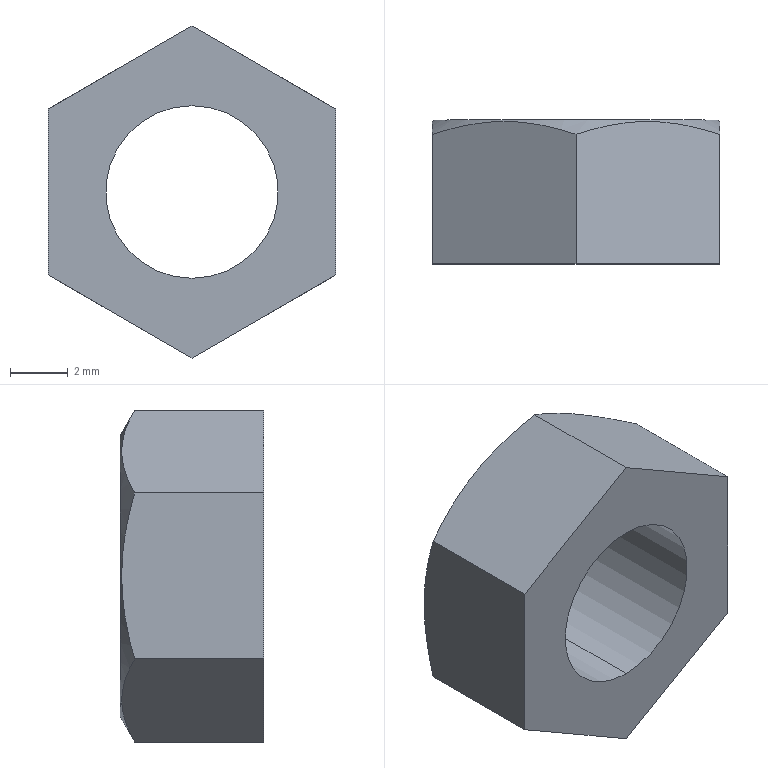Part | STEP file | NN42-M6 | 1 solid | 12 faces | box 10 x 5 x 11.547 mm | volume 289.993 mm3 | plane 8 | cylinder 2 | cone 2 | commonest cylinder face diameters 6 x2
STEP:
#1=CARTESIAN_POINT('',(0.,0.,0.));
#2=DIRECTION('',(0.,0.,1.));
#3=DIRECTION('',(1.,0.,0.));
#4=AXIS2_PLACEMENT_3D('',#1,#2,#3);
#5=CARTESIAN_POINT('',(0.,5.,-3.));
#6=VERTEX_POINT('',#5);
#7=CARTESIAN_POINT('',(0.,0.,-3.));
#8=VERTEX_POINT('',#7);
#9=CARTESIAN_POINT('',(0.,5.,-3.));
#10=DIRECTION('',(0.,-1.,0.));
#11=VECTOR('',#10,1.);
#12=LINE('',#9,#11);
#13=CARTESIAN_POINT('',(0.,5.,0.));
#14=DIRECTION('',(0.,-1.,0.));
#15=DIRECTION('',(0.,0.,-1.));
#16=AXIS2_PLACEMENT_3D('',#13,#14,#15);
#17=CYLINDRICAL_SURFACE('',#16,3.);
#18=CARTESIAN_POINT('',(6.283,0.));
#19=DIRECTION('',(0.,1.));
#20=VECTOR('',#19,1.);
#21=LINE('',#18,#20);
#22=(GEOMETRIC_REPRESENTATION_CONTEXT(2)PARAMETRIC_REPRESENTATION_CONTEXT()REPRESENTATION_CONTEXT('',''));
#23=DEFINITIONAL_REPRESENTATION('',(#21),#22);
#24=PCURVE('',#17,#23);
#25=CARTESIAN_POINT('',(0.,5.,0.));
#26=DIRECTION('',(0.,-1.,0.));
#27=DIRECTION('',(0.,0.,-1.));
#28=AXIS2_PLACEMENT_3D('',#25,#26,#27);
#29=CYLINDRICAL_SURFACE('',#28,3.);
#30=CARTESIAN_POINT('',(0.,0.));
#31=DIRECTION('',(0.,1.));
#32=VECTOR('',#31,1.);
#33=LINE('',#30,#32);
#34=(GEOMETRIC_REPRESENTATION_CONTEXT(2)PARAMETRIC_REPRESENTATION_CONTEXT()REPRESENTATION_CONTEXT('',''));
#35=DEFINITIONAL_REPRESENTATION('',(#33),#34);
#36=PCURVE('',#29,#35);
#37=SURFACE_CURVE('',#12,(#24,#36),.PCURVE_S1.);
#38=EDGE_CURVE('',#6,#8,#37,.T.);
#39=ORIENTED_EDGE('',*,*,#38,.T.);
#40=CARTESIAN_POINT('',(0.,0.,3.));
#41=VERTEX_POINT('',#40);
#42=CARTESIAN_POINT('',(0.,0.,0.));
#43=DIRECTION('',(0.,1.,0.));
#44=DIRECTION('',(0.,0.,1.));
#45=AXIS2_PLACEMENT_3D('',#42,#43,#44);
#46=CIRCLE('',#45,3.);
#47=CARTESIAN_POINT('',(9.425,5.));
#48=DIRECTION('',(-1.,0.));
#49=VECTOR('',#48,1.);
#50=LINE('',#47,#49);
#51=(GEOMETRIC_REPRESENTATION_CONTEXT(2)PARAMETRIC_REPRESENTATION_CONTEXT()REPRESENTATION_CONTEXT('',''));
#52=DEFINITIONAL_REPRESENTATION('',(#50),#51);
#53=PCURVE('',#17,#52);
#54=CARTESIAN_POINT('',(0.,0.,0.));
#55=DIRECTION('',(0.,-1.,0.));
#56=DIRECTION('',(0.,0.,1.));
#57=AXIS2_PLACEMENT_3D('',#54,#55,#56);
#58=PLANE('',#57);
#59=CARTESIAN_POINT('',(3.,0.));
#60=CARTESIAN_POINT('',(3.,-5.196));
#61=CARTESIAN_POINT('',(-1.5,-2.598));
#62=CARTESIAN_POINT('',(-6.,0.));
#63=CARTESIAN_POINT('',(-1.5,2.598));
#64=CARTESIAN_POINT('',(3.,5.196));
#65=CARTESIAN_POINT('',(3.,0.));
#66=(BOUNDED_CURVE()B_SPLINE_CURVE(2,(#59,#60,#61,#62,#63,#64,#65),.UNSPECIFIED.,.T.,.F.)B_SPLINE_CURVE_WITH_KNOTS((1,2,2,2,2,1),(-2.094,0.,2.094,4.189,6.283,8.378),.UNSPECIFIED.)CURVE()GEOMETRIC_REPRESENTATION_ITEM()RATIONAL_B_SPLINE_CURVE((1.,0.5,1.,0.5,1.,0.5,1.))REPRESENTATION_ITEM(''));
#67=(GEOMETRIC_REPRESENTATION_CONTEXT(2)PARAMETRIC_REPRESENTATION_CONTEXT()REPRESENTATION_CONTEXT('',''));
#68=DEFINITIONAL_REPRESENTATION('',(#66),#67);
#69=PCURVE('',#58,#68);
#70=SURFACE_CURVE('',#46,(#53,#69),.PCURVE_S1.);
#71=EDGE_CURVE('',#8,#41,#70,.T.);
#72=ORIENTED_EDGE('',*,*,#71,.T.);
#73=CARTESIAN_POINT('',(0.,5.,3.));
#74=VERTEX_POINT('',#73);
#75=CARTESIAN_POINT('',(0.,5.,3.));
#76=DIRECTION('',(0.,-1.,0.));
#77=VECTOR('',#76,1.);
#78=LINE('',#75,#77);
#79=CARTESIAN_POINT('',(3.142,0.));
#80=DIRECTION('',(0.,1.));
#81=VECTOR('',#80,1.);
#82=LINE('',#79,#81);
#83=(GEOMETRIC_REPRESENTATION_CONTEXT(2)PARAMETRIC_REPRESENTATION_CONTEXT()REPRESENTATION_CONTEXT('',''));
#84=DEFINITIONAL_REPRESENTATION('',(#82),#83);
#85=PCURVE('',#17,#84);
#86=CARTESIAN_POINT('',(3.142,0.));
#87=DIRECTION('',(0.,1.));
#88=VECTOR('',#87,1.);
#89=LINE('',#86,#88);
#90=(GEOMETRIC_REPRESENTATION_CONTEXT(2)PARAMETRIC_REPRESENTATION_CONTEXT()REPRESENTATION_CONTEXT('',''));
#91=DEFINITIONAL_REPRESENTATION('',(#89),#90);
#92=PCURVE('',#29,#91);
#93=SURFACE_CURVE('',#78,(#85,#92),.PCURVE_S1.);
#94=EDGE_CURVE('',#74,#41,#93,.T.);
#95=ORIENTED_EDGE('',*,*,#94,.F.);
#96=CARTESIAN_POINT('',(0.,5.,0.));
#97=DIRECTION('',(0.,-1.,0.));
#98=DIRECTION('',(0.,0.,-1.));
#99=AXIS2_PLACEMENT_3D('',#96,#97,#98);
#100=CIRCLE('',#99,3.);
#101=CARTESIAN_POINT('',(0.,0.));
#102=DIRECTION('',(1.,0.));
#103=VECTOR('',#102,1.);
#104=LINE('',#101,#103);
#105=(GEOMETRIC_REPRESENTATION_CONTEXT(2)PARAMETRIC_REPRESENTATION_CONTEXT()REPRESENTATION_CONTEXT('',''));
#106=DEFINITIONAL_REPRESENTATION('',(#104),#105);
#107=PCURVE('',#17,#106);
#108=CARTESIAN_POINT('',(0.,5.,0.));
#109=DIRECTION('',(0.,1.,0.));
#110=DIRECTION('',(-1.,0.,0.));
#111=AXIS2_PLACEMENT_3D('',#108,#109,#110);
#112=PLANE('',#111);
#113=CARTESIAN_POINT('',(0.,-3.));
#114=CARTESIAN_POINT('',(-5.196,-3.));
#115=CARTESIAN_POINT('',(-2.598,1.5));
#116=CARTESIAN_POINT('',(0.,6.));
#117=CARTESIAN_POINT('',(2.598,1.5));
#118=CARTESIAN_POINT('',(5.196,-3.));
#119=CARTESIAN_POINT('',(0.,-3.));
#120=(BOUNDED_CURVE()B_SPLINE_CURVE(2,(#113,#114,#115,#116,#117,#118,#119),.UNSPECIFIED.,.T.,.F.)B_SPLINE_CURVE_WITH_KNOTS((1,2,2,2,2,1),(-2.094,0.,2.094,4.189,6.283,8.378),.UNSPECIFIED.)CURVE()GEOMETRIC_REPRESENTATION_ITEM()RATIONAL_B_SPLINE_CURVE((1.,0.5,1.,0.5,1.,0.5,1.))REPRESENTATION_ITEM(''));
#121=(GEOMETRIC_REPRESENTATION_CONTEXT(2)PARAMETRIC_REPRESENTATION_CONTEXT()REPRESENTATION_CONTEXT('',''));
#122=DEFINITIONAL_REPRESENTATION('',(#120),#121);
#123=PCURVE('',#112,#122);
#124=SURFACE_CURVE('',#100,(#107,#123),.PCURVE_S1.);
#125=EDGE_CURVE('',#74,#6,#124,.T.);
#126=ORIENTED_EDGE('',*,*,#125,.T.);
#127=EDGE_LOOP('',(#39,#72,#95,#126));
#128=FACE_BOUND('',#127,.F.);
#129=ADVANCED_FACE('',(#128),#17,.F.);
#130=CARTESIAN_POINT('',(4.9,5.,0.));
#131=VERTEX_POINT('',#130);
#132=CARTESIAN_POINT('',(-4.9,5.,0.));
#133=VERTEX_POINT('',#132);
#134=CARTESIAN_POINT('',(0.,5.,0.));
#135=DIRECTION('',(0.,-1.,0.));
#136=DIRECTION('',(1.,0.,0.));
#137=AXIS2_PLACEMENT_3D('',#134,#135,#136);
#138=CIRCLE('',#137,4.9);
#139=CARTESIAN_POINT('',(0.,5.,0.));
#140=DIRECTION('',(0.,-1.,0.));
#141=DIRECTION('',(1.,0.,0.));
#142=AXIS2_PLACEMENT_3D('',#139,#140,#141);
#143=CONICAL_SURFACE('',#142,4.9,1.047);
#144=CARTESIAN_POINT('',(0.,0.));
#145=DIRECTION('',(1.,0.));
#146=VECTOR('',#145,1.);
#147=LINE('',#144,#146);
#148=(GEOMETRIC_REPRESENTATION_CONTEXT(2)PARAMETRIC_REPRESENTATION_CONTEXT()REPRESENTATION_CONTEXT('',''));
#149=DEFINITIONAL_REPRESENTATION('',(#147),#148);
#150=PCURVE('',#143,#149);
#151=CARTESIAN_POINT('',(-4.9,0.));
#152=CARTESIAN_POINT('',(-4.9,8.487));
#153=CARTESIAN_POINT('',(2.45,4.244));
#154=CARTESIAN_POINT('',(9.8,0.));
#155=CARTESIAN_POINT('',(2.45,-4.244));
#156=CARTESIAN_POINT('',(-4.9,-8.487));
#157=CARTESIAN_POINT('',(-4.9,0.));
#158=(BOUNDED_CURVE()B_SPLINE_CURVE(2,(#151,#152,#153,#154,#155,#156,#157),.UNSPECIFIED.,.T.,.F.)B_SPLINE_CURVE_WITH_KNOTS((1,2,2,2,2,1),(-2.094,0.,2.094,4.189,6.283,8.378),.UNSPECIFIED.)CURVE()GEOMETRIC_REPRESENTATION_ITEM()RATIONAL_B_SPLINE_CURVE((1.,0.5,1.,0.5,1.,0.5,1.))REPRESENTATION_ITEM(''));
#159=(GEOMETRIC_REPRESENTATION_CONTEXT(2)PARAMETRIC_REPRESENTATION_CONTEXT()REPRESENTATION_CONTEXT('',''));
#160=DEFINITIONAL_REPRESENTATION('',(#158),#159);
#161=PCURVE('',#112,#160);
#162=SURFACE_CURVE('',#138,(#150,#161),.PCURVE_S1.);
#163=EDGE_CURVE('',#131,#133,#162,.T.);
#164=ORIENTED_EDGE('',*,*,#163,.T.);
#165=CARTESIAN_POINT('',(-5.,4.942,0.));
#166=VERTEX_POINT('',#165);
#167=CARTESIAN_POINT('',(-4.9,5.,0.));
#168=DIRECTION('',(-0.866,-0.5,0.));
#169=VECTOR('',#168,1.);
#170=LINE('',#167,#169);
#171=CARTESIAN_POINT('',(3.142,0.));
#172=DIRECTION('',(0.,1.));
#173=VECTOR('',#172,1.);
#174=LINE('',#171,#173);
#175=(GEOMETRIC_REPRESENTATION_CONTEXT(2)PARAMETRIC_REPRESENTATION_CONTEXT()REPRESENTATION_CONTEXT('',''));
#176=DEFINITIONAL_REPRESENTATION('',(#174),#175);
#177=PCURVE('',#143,#176);
#178=CARTESIAN_POINT('',(0.,5.,0.));
#179=DIRECTION('',(0.,-1.,0.));
#180=DIRECTION('',(1.,0.,0.));
#181=AXIS2_PLACEMENT_3D('',#178,#179,#180);
#182=CONICAL_SURFACE('',#181,4.9,1.047);
#183=CARTESIAN_POINT('',(3.142,0.));
#184=DIRECTION('',(0.,1.));
#185=VECTOR('',#184,1.);
#186=LINE('',#183,#185);
#187=(GEOMETRIC_REPRESENTATION_CONTEXT(2)PARAMETRIC_REPRESENTATION_CONTEXT()REPRESENTATION_CONTEXT('',''));
#188=DEFINITIONAL_REPRESENTATION('',(#186),#187);
#189=PCURVE('',#182,#188);
#190=SURFACE_CURVE('',#170,(#177,#189),.PCURVE_S1.);
#191=EDGE_CURVE('',#133,#166,#190,.T.);
#192=ORIENTED_EDGE('',*,*,#191,.T.);
#193=CARTESIAN_POINT('',(-5.,4.496,2.887));
#194=VERTEX_POINT('',#193);
#195=CARTESIAN_POINT('',(-5.,4.496,2.887));
#196=CARTESIAN_POINT('',(-5.,4.767,1.946));
#197=CARTESIAN_POINT('',(-5.,4.942,0.9887));
#198=CARTESIAN_POINT('',(-5.,4.942,0.));
#199=B_SPLINE_CURVE_WITH_KNOTS('',3,(#195,#196,#197,#198),.UNSPECIFIED.,.F.,.F.,(4,4),(0.006295,0.009232),.PIECEWISE_BEZIER_KNOTS.);
#200=CARTESIAN_POINT('',(2.618,0.5043));
#201=CARTESIAN_POINT('',(2.624,0.492));
#202=CARTESIAN_POINT('',(2.637,0.4677));
#203=CARTESIAN_POINT('',(2.657,0.4325));
#204=CARTESIAN_POINT('',(2.678,0.3985));
#205=CARTESIAN_POINT('',(2.699,0.3659));
#206=CARTESIAN_POINT('',(2.72,0.3347));
#207=CARTESIAN_POINT('',(2.742,0.3048));
#208=CARTESIAN_POINT('',(2.764,0.2764));
#209=CARTESIAN_POINT('',(2.787,0.2495));
#210=CARTESIAN_POINT('',(2.81,0.2242));
#211=CARTESIAN_POINT('',(2.833,0.2005));
#212=CARTESIAN_POINT('',(2.857,0.1784));
#213=CARTESIAN_POINT('',(2.882,0.158));
#214=CARTESIAN_POINT('',(2.906,0.1394));
#215=CARTESIAN_POINT('',(2.931,0.1226));
#216=CARTESIAN_POINT('',(2.957,0.1076));
#217=CARTESIAN_POINT('',(2.982,0.09448));
#218=CARTESIAN_POINT('',(3.008,0.08328));
#219=CARTESIAN_POINT('',(3.035,0.07404));
#220=CARTESIAN_POINT('',(3.061,0.0668));
#221=CARTESIAN_POINT('',(3.088,0.06159));
#222=CARTESIAN_POINT('',(3.115,0.05844));
#223=CARTESIAN_POINT('',(3.133,0.05773));
#224=CARTESIAN_POINT('',(3.142,0.05774));
#225=B_SPLINE_CURVE_WITH_KNOTS('',3,(#200,#201,#202,#203,#204,#205,#206,#207,#208,#209,#210,#211,#212,#213,#214,#215,#216,#217,#218,#219,#220,#221,#222,#223,#224),.UNSPECIFIED.,.F.,.F.,(4,1,1,1,1,1,1,1,1,1,1,1,1,1,1,1,1,1,1,1,1,1,4),(0.006295,0.006428,0.006562,0.006695,0.006829,0.006962,0.007096,0.007229,0.007363,0.007496,0.00763,0.007763,0.007897,0.00803,0.008164,0.008297,0.008431,0.008564,0.008698,0.008831,0.008965,0.009098,0.009232),.QUASI_UNIFORM_KNOTS.);
#226=(GEOMETRIC_REPRESENTATION_CONTEXT(2)PARAMETRIC_REPRESENTATION_CONTEXT()REPRESENTATION_CONTEXT('',''));
#227=DEFINITIONAL_REPRESENTATION('',(#225),#226);
#228=PCURVE('',#143,#227);
#229=CARTESIAN_POINT('',(-5.,4.496,2.887));
#230=DIRECTION('',(1.,0.,0.));
#231=DIRECTION('',(0.,0.,1.));
#232=AXIS2_PLACEMENT_3D('',#229,#230,#231);
#233=PLANE('',#232);
#234=CARTESIAN_POINT('',(0.,0.));
#235=CARTESIAN_POINT('',(-0.9405,-0.2715));
#236=CARTESIAN_POINT('',(-1.898,-0.4466));
#237=CARTESIAN_POINT('',(-2.887,-0.4466));
#238=B_SPLINE_CURVE_WITH_KNOTS('',3,(#234,#235,#236,#237),.UNSPECIFIED.,.F.,.F.,(4,4),(0.006295,0.009232),.PIECEWISE_BEZIER_KNOTS.);
#239=(GEOMETRIC_REPRESENTATION_CONTEXT(2)PARAMETRIC_REPRESENTATION_CONTEXT()REPRESENTATION_CONTEXT('',''));
#240=DEFINITIONAL_REPRESENTATION('',(#238),#239);
#241=PCURVE('',#233,#240);
#242=SURFACE_CURVE('',#199,(#228,#241),.PCURVE_S1.);
#243=EDGE_CURVE('',#194,#166,#242,.T.);
#244=ORIENTED_EDGE('',*,*,#243,.F.);
#245=CARTESIAN_POINT('',(0.,4.496,5.774));
#246=VERTEX_POINT('',#245);
#247=CARTESIAN_POINT('',(0.,4.496,5.774));
#248=CARTESIAN_POINT('',(-0.8164,4.768,5.302));
#249=CARTESIAN_POINT('',(-1.645,4.942,4.824));
#250=CARTESIAN_POINT('',(-2.708,4.942,4.21));
#251=CARTESIAN_POINT('',(-2.921,4.932,4.087));
#252=CARTESIAN_POINT('',(-3.344,4.891,3.843));
#253=CARTESIAN_POINT('',(-3.554,4.861,3.722));
#254=CARTESIAN_POINT('',(-4.179,4.744,3.361));
#255=CARTESIAN_POINT('',(-4.591,4.632,3.123));
#256=CARTESIAN_POINT('',(-5.,4.496,2.887));
#257=B_SPLINE_CURVE_WITH_KNOTS('',3,(#247,#248,#249,#250,#251,#252,#253,#254,#255,#256),.UNSPECIFIED.,.F.,.F.,(4,2,2,2,4),(0.000000238,0.002916,0.003645,0.004373,0.005831),.UNSPECIFIED.);
#258=CARTESIAN_POINT('',(1.571,0.5043));
#259=CARTESIAN_POINT('',(1.584,0.4796));
#260=CARTESIAN_POINT('',(1.61,0.4317));
#261=CARTESIAN_POINT('',(1.651,0.365));
#262=CARTESIAN_POINT('',(1.694,0.3038));
#263=CARTESIAN_POINT('',(1.739,0.2486));
#264=CARTESIAN_POINT('',(1.786,0.1995));
#265=CARTESIAN_POINT('',(1.834,0.1571));
#266=CARTESIAN_POINT('',(1.884,0.1217));
#267=CARTESIAN_POINT('',(1.935,0.09364));
#268=CARTESIAN_POINT('',(1.987,0.07321));
#269=CARTESIAN_POINT('',(2.04,0.06069));
#270=CARTESIAN_POINT('',(2.093,0.05635));
#271=CARTESIAN_POINT('',(2.147,0.06034));
#272=CARTESIAN_POINT('',(2.2,0.07259));
#273=CARTESIAN_POINT('',(2.253,0.09288));
#274=CARTESIAN_POINT('',(2.304,0.1209));
#275=CARTESIAN_POINT('',(2.354,0.1563));
#276=CARTESIAN_POINT('',(2.402,0.1988));
#277=CARTESIAN_POINT('',(2.449,0.248));
#278=CARTESIAN_POINT('',(2.494,0.3034));
#279=CARTESIAN_POINT('',(2.537,0.3648));
#280=CARTESIAN_POINT('',(2.579,0.4316));
#281=CARTESIAN_POINT('',(2.605,0.4795));
#282=CARTESIAN_POINT('',(2.618,0.5043));
#283=B_SPLINE_CURVE_WITH_KNOTS('',3,(#258,#259,#260,#261,#262,#263,#264,#265,#266,#267,#268,#269,#270,#271,#272,#273,#274,#275,#276,#277,#278,#279,#280,#281,#282),.UNSPECIFIED.,.F.,.F.,(4,1,1,1,1,1,1,1,1,1,1,1,1,1,1,1,1,1,1,1,1,1,4),(0.000000238,0.0002653,0.0005303,0.0007954,0.00106,0.001325,0.00159,0.001856,0.002121,0.002386,0.002651,0.002916,0.003181,0.003446,0.003711,0.003976,0.004241,0.004506,0.004771,0.005036,0.005301,0.005566,0.005831),.QUASI_UNIFORM_KNOTS.);
#284=(GEOMETRIC_REPRESENTATION_CONTEXT(2)PARAMETRIC_REPRESENTATION_CONTEXT()REPRESENTATION_CONTEXT('',''));
#285=DEFINITIONAL_REPRESENTATION('',(#283),#284);
#286=PCURVE('',#143,#285);
#287=CARTESIAN_POINT('',(0.,4.496,5.774));
#288=DIRECTION('',(0.5,0.,-0.866));
#289=DIRECTION('',(0.866,0.,0.5));
#290=AXIS2_PLACEMENT_3D('',#287,#288,#289);
#291=PLANE('',#290);
#292=CARTESIAN_POINT('',(0.,0.));
#293=CARTESIAN_POINT('',(-0.9427,-0.2721));
#294=CARTESIAN_POINT('',(-1.9,-0.446));
#295=CARTESIAN_POINT('',(-3.127,-0.4467));
#296=CARTESIAN_POINT('',(-3.373,-0.4363));
#297=CARTESIAN_POINT('',(-3.861,-0.3956));
#298=CARTESIAN_POINT('',(-4.103,-0.3654));
#299=CARTESIAN_POINT('',(-4.826,-0.2487));
#300=CARTESIAN_POINT('',(-5.302,-0.1362));
#301=CARTESIAN_POINT('',(-5.774,0.));
#302=B_SPLINE_CURVE_WITH_KNOTS('',3,(#292,#293,#294,#295,#296,#297,#298,#299,#300,#301),.UNSPECIFIED.,.F.,.F.,(4,2,2,2,4),(0.000000238,0.002916,0.003645,0.004373,0.005831),.UNSPECIFIED.);
#303=(GEOMETRIC_REPRESENTATION_CONTEXT(2)PARAMETRIC_REPRESENTATION_CONTEXT()REPRESENTATION_CONTEXT('',''));
#304=DEFINITIONAL_REPRESENTATION('',(#302),#303);
#305=PCURVE('',#291,#304);
#306=SURFACE_CURVE('',#257,(#286,#305),.PCURVE_S1.);
#307=EDGE_CURVE('',#246,#194,#306,.T.);
#308=ORIENTED_EDGE('',*,*,#307,.F.);
#309=CARTESIAN_POINT('',(5.,4.496,2.887));
#310=VERTEX_POINT('',#309);
#311=CARTESIAN_POINT('',(5.,4.496,2.887));
#312=CARTESIAN_POINT('',(4.184,4.768,3.358));
#313=CARTESIAN_POINT('',(3.355,4.942,3.837));
#314=CARTESIAN_POINT('',(2.292,4.942,4.45));
#315=CARTESIAN_POINT('',(2.079,4.932,4.573));
#316=CARTESIAN_POINT('',(1.656,4.891,4.817));
#317=CARTESIAN_POINT('',(1.446,4.861,4.938));
#318=CARTESIAN_POINT('',(0.8208,4.744,5.3));
#319=CARTESIAN_POINT('',(0.4087,4.632,5.538));
#320=CARTESIAN_POINT('',(0.,4.496,5.774));
#321=B_SPLINE_CURVE_WITH_KNOTS('',3,(#311,#312,#313,#314,#315,#316,#317,#318,#319,#320),.UNSPECIFIED.,.F.,.F.,(4,2,2,2,4),(0.000000238,0.002916,0.003645,0.004373,0.005831),.UNSPECIFIED.);
#322=CARTESIAN_POINT('',(0.5236,0.5043));
#323=CARTESIAN_POINT('',(0.5365,0.4796));
#324=CARTESIAN_POINT('',(0.5628,0.4317));
#325=CARTESIAN_POINT('',(0.6041,0.365));
#326=CARTESIAN_POINT('',(0.6472,0.3038));
#327=CARTESIAN_POINT('',(0.6921,0.2486));
#328=CARTESIAN_POINT('',(0.7388,0.1995));
#329=CARTESIAN_POINT('',(0.787,0.1571));
#330=CARTESIAN_POINT('',(0.8367,0.1217));
#331=CARTESIAN_POINT('',(0.8877,0.09364));
#332=CARTESIAN_POINT('',(0.9398,0.07321));
#333=CARTESIAN_POINT('',(0.9926,0.06069));
#334=CARTESIAN_POINT('',(1.046,0.05635));
#335=CARTESIAN_POINT('',(1.1,0.06034));
#336=CARTESIAN_POINT('',(1.153,0.07259));
#337=CARTESIAN_POINT('',(1.205,0.09288));
#338=CARTESIAN_POINT('',(1.257,0.1209));
#339=CARTESIAN_POINT('',(1.307,0.1563));
#340=CARTESIAN_POINT('',(1.355,0.1988));
#341=CARTESIAN_POINT('',(1.402,0.248));
#342=CARTESIAN_POINT('',(1.447,0.3034));
#343=CARTESIAN_POINT('',(1.49,0.3648));
#344=CARTESIAN_POINT('',(1.532,0.4316));
#345=CARTESIAN_POINT('',(1.558,0.4795));
#346=CARTESIAN_POINT('',(1.571,0.5043));
#347=B_SPLINE_CURVE_WITH_KNOTS('',3,(#322,#323,#324,#325,#326,#327,#328,#329,#330,#331,#332,#333,#334,#335,#336,#337,#338,#339,#340,#341,#342,#343,#344,#345,#346),.UNSPECIFIED.,.F.,.F.,(4,1,1,1,1,1,1,1,1,1,1,1,1,1,1,1,1,1,1,1,1,1,4),(0.000000238,0.0002653,0.0005303,0.0007954,0.00106,0.001325,0.00159,0.001856,0.002121,0.002386,0.002651,0.002916,0.003181,0.003446,0.003711,0.003976,0.004241,0.004506,0.004771,0.005036,0.005301,0.005566,0.005831),.QUASI_UNIFORM_KNOTS.);
#348=(GEOMETRIC_REPRESENTATION_CONTEXT(2)PARAMETRIC_REPRESENTATION_CONTEXT()REPRESENTATION_CONTEXT('',''));
#349=DEFINITIONAL_REPRESENTATION('',(#347),#348);
#350=PCURVE('',#143,#349);
#351=CARTESIAN_POINT('',(5.,4.496,2.887));
#352=DIRECTION('',(-0.5,0.,-0.866));
#353=DIRECTION('',(0.866,0.,-0.5));
#354=AXIS2_PLACEMENT_3D('',#351,#352,#353);
#355=PLANE('',#354);
#356=CARTESIAN_POINT('',(0.,0.));
#357=CARTESIAN_POINT('',(-0.9427,-0.2721));
#358=CARTESIAN_POINT('',(-1.9,-0.446));
#359=CARTESIAN_POINT('',(-3.127,-0.4467));
#360=CARTESIAN_POINT('',(-3.373,-0.4363));
#361=CARTESIAN_POINT('',(-3.861,-0.3956));
#362=CARTESIAN_POINT('',(-4.103,-0.3654));
#363=CARTESIAN_POINT('',(-4.826,-0.2487));
#364=CARTESIAN_POINT('',(-5.302,-0.1362));
#365=CARTESIAN_POINT('',(-5.774,0.));
#366=B_SPLINE_CURVE_WITH_KNOTS('',3,(#356,#357,#358,#359,#360,#361,#362,#363,#364,#365),.UNSPECIFIED.,.F.,.F.,(4,2,2,2,4),(0.000000238,0.002916,0.003645,0.004373,0.005831),.UNSPECIFIED.);
#367=(GEOMETRIC_REPRESENTATION_CONTEXT(2)PARAMETRIC_REPRESENTATION_CONTEXT()REPRESENTATION_CONTEXT('',''));
#368=DEFINITIONAL_REPRESENTATION('',(#366),#367);
#369=PCURVE('',#355,#368);
#370=SURFACE_CURVE('',#321,(#350,#369),.PCURVE_S1.);
#371=EDGE_CURVE('',#310,#246,#370,.T.);
#372=ORIENTED_EDGE('',*,*,#371,.F.);
#373=CARTESIAN_POINT('',(5.,4.942,0.));
#374=VERTEX_POINT('',#373);
#375=CARTESIAN_POINT('',(5.,4.942,0.));
#376=CARTESIAN_POINT('',(5.,4.942,0.4941));
#377=CARTESIAN_POINT('',(5.,4.899,0.982));
#378=CARTESIAN_POINT('',(5.,4.743,1.943));
#379=CARTESIAN_POINT('',(5.,4.631,2.417));
#380=CARTESIAN_POINT('',(5.,4.496,2.887));
#381=B_SPLINE_CURVE_WITH_KNOTS('',3,(#375,#376,#377,#378,#379,#380),.UNSPECIFIED.,.F.,.F.,(4,2,4),(0.009232,0.0107,0.01217),.UNSPECIFIED.);
#382=CARTESIAN_POINT('',(0.,0.05774));
#383=CARTESIAN_POINT('',(0.008983,0.05773));
#384=CARTESIAN_POINT('',(0.02693,0.05844));
#385=CARTESIAN_POINT('',(0.05375,0.06158));
#386=CARTESIAN_POINT('',(0.08042,0.06677));
#387=CARTESIAN_POINT('',(0.1069,0.074));
#388=CARTESIAN_POINT('',(0.1332,0.08323));
#389=CARTESIAN_POINT('',(0.1592,0.09442));
#390=CARTESIAN_POINT('',(0.185,0.1075));
#391=CARTESIAN_POINT('',(0.2104,0.1225));
#392=CARTESIAN_POINT('',(0.2355,0.1394));
#393=CARTESIAN_POINT('',(0.2603,0.158));
#394=CARTESIAN_POINT('',(0.2846,0.1784));
#395=CARTESIAN_POINT('',(0.3086,0.2005));
#396=CARTESIAN_POINT('',(0.3321,0.2242));
#397=CARTESIAN_POINT('',(0.3552,0.2496));
#398=CARTESIAN_POINT('',(0.3779,0.2765));
#399=CARTESIAN_POINT('',(0.4001,0.3049));
#400=CARTESIAN_POINT('',(0.4218,0.3347));
#401=CARTESIAN_POINT('',(0.4431,0.366));
#402=CARTESIAN_POINT('',(0.464,0.3986));
#403=CARTESIAN_POINT('',(0.4843,0.4325));
#404=CARTESIAN_POINT('',(0.5042,0.4677));
#405=CARTESIAN_POINT('',(0.5172,0.492));
#406=CARTESIAN_POINT('',(0.5236,0.5043));
#407=B_SPLINE_CURVE_WITH_KNOTS('',3,(#382,#383,#384,#385,#386,#387,#388,#389,#390,#391,#392,#393,#394,#395,#396,#397,#398,#399,#400,#401,#402,#403,#404,#405,#406),.UNSPECIFIED.,.F.,.F.,(4,1,1,1,1,1,1,1,1,1,1,1,1,1,1,1,1,1,1,1,1,1,4),(0.009232,0.009365,0.009499,0.009632,0.009765,0.009899,0.01003,0.01017,0.0103,0.01043,0.01057,0.0107,0.01083,0.01097,0.0111,0.01123,0.01137,0.0115,0.01163,0.01177,0.0119,0.01203,0.01217),.QUASI_UNIFORM_KNOTS.);
#408=(GEOMETRIC_REPRESENTATION_CONTEXT(2)PARAMETRIC_REPRESENTATION_CONTEXT()REPRESENTATION_CONTEXT('',''));
#409=DEFINITIONAL_REPRESENTATION('',(#407),#408);
#410=PCURVE('',#143,#409);
#411=CARTESIAN_POINT('',(5.,4.496,-2.887));
#412=DIRECTION('',(-1.,0.,0.));
#413=DIRECTION('',(0.,0.,-1.));
#414=AXIS2_PLACEMENT_3D('',#411,#412,#413);
#415=PLANE('',#414);
#416=CARTESIAN_POINT('',(-2.887,-0.4466));
#417=CARTESIAN_POINT('',(-3.381,-0.4466));
#418=CARTESIAN_POINT('',(-3.869,-0.4035));
#419=CARTESIAN_POINT('',(-4.83,-0.2477));
#420=CARTESIAN_POINT('',(-5.304,-0.1356));
#421=CARTESIAN_POINT('',(-5.774,0.));
#422=B_SPLINE_CURVE_WITH_KNOTS('',3,(#416,#417,#418,#419,#420,#421),.UNSPECIFIED.,.F.,.F.,(4,2,4),(0.009232,0.0107,0.01217),.UNSPECIFIED.);
#423=(GEOMETRIC_REPRESENTATION_CONTEXT(2)PARAMETRIC_REPRESENTATION_CONTEXT()REPRESENTATION_CONTEXT('',''));
#424=DEFINITIONAL_REPRESENTATION('',(#422),#423);
#425=PCURVE('',#415,#424);
#426=SURFACE_CURVE('',#381,(#410,#425),.PCURVE_S1.);
#427=EDGE_CURVE('',#374,#310,#426,.T.);
#428=ORIENTED_EDGE('',*,*,#427,.F.);
#429=CARTESIAN_POINT('',(4.9,5.,0.));
#430=DIRECTION('',(0.866,-0.5,0.));
#431=VECTOR('',#430,1.);
#432=LINE('',#429,#431);
#433=CARTESIAN_POINT('',(0.,0.));
#434=DIRECTION('',(0.,1.));
#435=VECTOR('',#434,1.);
#436=LINE('',#433,#435);
#437=(GEOMETRIC_REPRESENTATION_CONTEXT(2)PARAMETRIC_REPRESENTATION_CONTEXT()REPRESENTATION_CONTEXT('',''));
#438=DEFINITIONAL_REPRESENTATION('',(#436),#437);
#439=PCURVE('',#143,#438);
#440=CARTESIAN_POINT('',(6.283,0.));
#441=DIRECTION('',(0.,1.));
#442=VECTOR('',#441,1.);
#443=LINE('',#440,#442);
#444=(GEOMETRIC_REPRESENTATION_CONTEXT(2)PARAMETRIC_REPRESENTATION_CONTEXT()REPRESENTATION_CONTEXT('',''));
#445=DEFINITIONAL_REPRESENTATION('',(#443),#444);
#446=PCURVE('',#182,#445);
#447=SURFACE_CURVE('',#432,(#439,#446),.PCURVE_S1.);
#448=EDGE_CURVE('',#131,#374,#447,.T.);
#449=ORIENTED_EDGE('',*,*,#448,.F.);
#450=EDGE_LOOP('',(#164,#192,#244,#308,#372,#428,#449));
#451=FACE_BOUND('',#450,.T.);
#452=ADVANCED_FACE('',(#451),#143,.T.);
#453=ORIENTED_EDGE('',*,*,#191,.F.);
#454=CARTESIAN_POINT('',(0.,5.,0.));
#455=DIRECTION('',(0.,-1.,0.));
#456=DIRECTION('',(1.,0.,0.));
#457=AXIS2_PLACEMENT_3D('',#454,#455,#456);
#458=CIRCLE('',#457,4.9);
#459=CARTESIAN_POINT('',(0.,0.));
#460=DIRECTION('',(1.,0.));
#461=VECTOR('',#460,1.);
#462=LINE('',#459,#461);
#463=(GEOMETRIC_REPRESENTATION_CONTEXT(2)PARAMETRIC_REPRESENTATION_CONTEXT()REPRESENTATION_CONTEXT('',''));
#464=DEFINITIONAL_REPRESENTATION('',(#462),#463);
#465=PCURVE('',#182,#464);
#466=CARTESIAN_POINT('',(-4.9,0.));
#467=CARTESIAN_POINT('',(-4.9,8.487));
#468=CARTESIAN_POINT('',(2.45,4.244));
#469=CARTESIAN_POINT('',(9.8,0.));
#470=CARTESIAN_POINT('',(2.45,-4.244));
#471=CARTESIAN_POINT('',(-4.9,-8.487));
#472=CARTESIAN_POINT('',(-4.9,0.));
#473=(BOUNDED_CURVE()B_SPLINE_CURVE(2,(#466,#467,#468,#469,#470,#471,#472),.UNSPECIFIED.,.T.,.F.)B_SPLINE_CURVE_WITH_KNOTS((1,2,2,2,2,1),(-2.094,0.,2.094,4.189,6.283,8.378),.UNSPECIFIED.)CURVE()GEOMETRIC_REPRESENTATION_ITEM()RATIONAL_B_SPLINE_CURVE((1.,0.5,1.,0.5,1.,0.5,1.))REPRESENTATION_ITEM(''));
#474=(GEOMETRIC_REPRESENTATION_CONTEXT(2)PARAMETRIC_REPRESENTATION_CONTEXT()REPRESENTATION_CONTEXT('',''));
#475=DEFINITIONAL_REPRESENTATION('',(#473),#474);
#476=PCURVE('',#112,#475);
#477=SURFACE_CURVE('',#458,(#465,#476),.PCURVE_S1.);
#478=EDGE_CURVE('',#133,#131,#477,.T.);
#479=ORIENTED_EDGE('',*,*,#478,.T.);
#480=ORIENTED_EDGE('',*,*,#448,.T.);
#481=CARTESIAN_POINT('',(5.,4.496,-2.887));
#482=VERTEX_POINT('',#481);
#483=CARTESIAN_POINT('',(5.,4.496,-2.887));
#484=CARTESIAN_POINT('',(5.,4.767,-1.946));
#485=CARTESIAN_POINT('',(5.,4.942,-0.9887));
#486=CARTESIAN_POINT('',(5.,4.942,0.));
#487=B_SPLINE_CURVE_WITH_KNOTS('',3,(#483,#484,#485,#486),.UNSPECIFIED.,.F.,.F.,(4,4),(0.006295,0.009232),.PIECEWISE_BEZIER_KNOTS.);
#488=CARTESIAN_POINT('',(5.76,0.5043));
#489=CARTESIAN_POINT('',(5.766,0.492));
#490=CARTESIAN_POINT('',(5.779,0.4677));
#491=CARTESIAN_POINT('',(5.799,0.4325));
#492=CARTESIAN_POINT('',(5.819,0.3985));
#493=CARTESIAN_POINT('',(5.84,0.3659));
#494=CARTESIAN_POINT('',(5.861,0.3347));
#495=CARTESIAN_POINT('',(5.883,0.3048));
#496=CARTESIAN_POINT('',(5.905,0.2764));
#497=CARTESIAN_POINT('',(5.928,0.2495));
#498=CARTESIAN_POINT('',(5.951,0.2242));
#499=CARTESIAN_POINT('',(5.975,0.2005));
#500=CARTESIAN_POINT('',(5.999,0.1784));
#501=CARTESIAN_POINT('',(6.023,0.158));
#502=CARTESIAN_POINT('',(6.048,0.1394));
#503=CARTESIAN_POINT('',(6.073,0.1226));
#504=CARTESIAN_POINT('',(6.098,0.1076));
#505=CARTESIAN_POINT('',(6.124,0.09448));
#506=CARTESIAN_POINT('',(6.15,0.08328));
#507=CARTESIAN_POINT('',(6.176,0.07404));
#508=CARTESIAN_POINT('',(6.203,0.0668));
#509=CARTESIAN_POINT('',(6.229,0.06159));
#510=CARTESIAN_POINT('',(6.256,0.05844));
#511=CARTESIAN_POINT('',(6.274,0.05773));
#512=CARTESIAN_POINT('',(6.283,0.05774));
#513=B_SPLINE_CURVE_WITH_KNOTS('',3,(#488,#489,#490,#491,#492,#493,#494,#495,#496,#497,#498,#499,#500,#501,#502,#503,#504,#505,#506,#507,#508,#509,#510,#511,#512),.UNSPECIFIED.,.F.,.F.,(4,1,1,1,1,1,1,1,1,1,1,1,1,1,1,1,1,1,1,1,1,1,4),(0.006295,0.006428,0.006562,0.006695,0.006829,0.006962,0.007096,0.007229,0.007363,0.007496,0.00763,0.007763,0.007897,0.00803,0.008164,0.008297,0.008431,0.008564,0.008698,0.008831,0.008965,0.009098,0.009232),.QUASI_UNIFORM_KNOTS.);
#514=(GEOMETRIC_REPRESENTATION_CONTEXT(2)PARAMETRIC_REPRESENTATION_CONTEXT()REPRESENTATION_CONTEXT('',''));
#515=DEFINITIONAL_REPRESENTATION('',(#513),#514);
#516=PCURVE('',#182,#515);
#517=CARTESIAN_POINT('',(0.,0.));
#518=CARTESIAN_POINT('',(-0.9405,-0.2715));
#519=CARTESIAN_POINT('',(-1.898,-0.4466));
#520=CARTESIAN_POINT('',(-2.887,-0.4466));
#521=B_SPLINE_CURVE_WITH_KNOTS('',3,(#517,#518,#519,#520),.UNSPECIFIED.,.F.,.F.,(4,4),(0.006295,0.009232),.PIECEWISE_BEZIER_KNOTS.);
#522=(GEOMETRIC_REPRESENTATION_CONTEXT(2)PARAMETRIC_REPRESENTATION_CONTEXT()REPRESENTATION_CONTEXT('',''));
#523=DEFINITIONAL_REPRESENTATION('',(#521),#522);
#524=PCURVE('',#415,#523);
#525=SURFACE_CURVE('',#487,(#516,#524),.PCURVE_S1.);
#526=EDGE_CURVE('',#482,#374,#525,.T.);
#527=ORIENTED_EDGE('',*,*,#526,.F.);
#528=CARTESIAN_POINT('',(0.,4.496,-5.774));
#529=VERTEX_POINT('',#528);
#530=CARTESIAN_POINT('',(0.,4.496,-5.774));
#531=CARTESIAN_POINT('',(0.8164,4.768,-5.302));
#532=CARTESIAN_POINT('',(1.645,4.942,-4.824));
#533=CARTESIAN_POINT('',(2.708,4.942,-4.21));
#534=CARTESIAN_POINT('',(2.921,4.932,-4.087));
#535=CARTESIAN_POINT('',(3.344,4.891,-3.843));
#536=CARTESIAN_POINT('',(3.554,4.861,-3.722));
#537=CARTESIAN_POINT('',(4.179,4.744,-3.361));
#538=CARTESIAN_POINT('',(4.591,4.632,-3.123));
#539=CARTESIAN_POINT('',(5.,4.496,-2.887));
#540=B_SPLINE_CURVE_WITH_KNOTS('',3,(#530,#531,#532,#533,#534,#535,#536,#537,#538,#539),.UNSPECIFIED.,.F.,.F.,(4,2,2,2,4),(0.000000238,0.002916,0.003645,0.004373,0.005831),.UNSPECIFIED.);
#541=CARTESIAN_POINT('',(4.712,0.5043));
#542=CARTESIAN_POINT('',(4.725,0.4796));
#543=CARTESIAN_POINT('',(4.752,0.4317));
#544=CARTESIAN_POINT('',(4.793,0.365));
#545=CARTESIAN_POINT('',(4.836,0.3038));
#546=CARTESIAN_POINT('',(4.881,0.2486));
#547=CARTESIAN_POINT('',(4.928,0.1995));
#548=CARTESIAN_POINT('',(4.976,0.1571));
#549=CARTESIAN_POINT('',(5.026,0.1217));
#550=CARTESIAN_POINT('',(5.076,0.09364));
#551=CARTESIAN_POINT('',(5.129,0.07321));
#552=CARTESIAN_POINT('',(5.181,0.06069));
#553=CARTESIAN_POINT('',(5.235,0.05635));
#554=CARTESIAN_POINT('',(5.288,0.06034));
#555=CARTESIAN_POINT('',(5.342,0.07259));
#556=CARTESIAN_POINT('',(5.394,0.09288));
#557=CARTESIAN_POINT('',(5.445,0.1209));
#558=CARTESIAN_POINT('',(5.495,0.1563));
#559=CARTESIAN_POINT('',(5.544,0.1988));
#560=CARTESIAN_POINT('',(5.591,0.248));
#561=CARTESIAN_POINT('',(5.636,0.3034));
#562=CARTESIAN_POINT('',(5.679,0.3648));
#563=CARTESIAN_POINT('',(5.72,0.4316));
#564=CARTESIAN_POINT('',(5.747,0.4795));
#565=CARTESIAN_POINT('',(5.76,0.5043));
#566=B_SPLINE_CURVE_WITH_KNOTS('',3,(#541,#542,#543,#544,#545,#546,#547,#548,#549,#550,#551,#552,#553,#554,#555,#556,#557,#558,#559,#560,#561,#562,#563,#564,#565),.UNSPECIFIED.,.F.,.F.,(4,1,1,1,1,1,1,1,1,1,1,1,1,1,1,1,1,1,1,1,1,1,4),(0.000000238,0.0002653,0.0005303,0.0007954,0.00106,0.001325,0.00159,0.001856,0.002121,0.002386,0.002651,0.002916,0.003181,0.003446,0.003711,0.003976,0.004241,0.004506,0.004771,0.005036,0.005301,0.005566,0.005831),.QUASI_UNIFORM_KNOTS.);
#567=(GEOMETRIC_REPRESENTATION_CONTEXT(2)PARAMETRIC_REPRESENTATION_CONTEXT()REPRESENTATION_CONTEXT('',''));
#568=DEFINITIONAL_REPRESENTATION('',(#566),#567);
#569=PCURVE('',#182,#568);
#570=CARTESIAN_POINT('',(0.,4.496,-5.774));
#571=DIRECTION('',(-0.5,0.,0.866));
#572=DIRECTION('',(-0.866,0.,-0.5));
#573=AXIS2_PLACEMENT_3D('',#570,#571,#572);
#574=PLANE('',#573);
#575=CARTESIAN_POINT('',(0.,0.));
#576=CARTESIAN_POINT('',(-0.9427,-0.2721));
#577=CARTESIAN_POINT('',(-1.9,-0.446));
#578=CARTESIAN_POINT('',(-3.127,-0.4467));
#579=CARTESIAN_POINT('',(-3.373,-0.4363));
#580=CARTESIAN_POINT('',(-3.861,-0.3956));
#581=CARTESIAN_POINT('',(-4.103,-0.3654));
#582=CARTESIAN_POINT('',(-4.826,-0.2487));
#583=CARTESIAN_POINT('',(-5.302,-0.1362));
#584=CARTESIAN_POINT('',(-5.774,0.));
#585=B_SPLINE_CURVE_WITH_KNOTS('',3,(#575,#576,#577,#578,#579,#580,#581,#582,#583,#584),.UNSPECIFIED.,.F.,.F.,(4,2,2,2,4),(0.000000238,0.002916,0.003645,0.004373,0.005831),.UNSPECIFIED.);
#586=(GEOMETRIC_REPRESENTATION_CONTEXT(2)PARAMETRIC_REPRESENTATION_CONTEXT()REPRESENTATION_CONTEXT('',''));
#587=DEFINITIONAL_REPRESENTATION('',(#585),#586);
#588=PCURVE('',#574,#587);
#589=SURFACE_CURVE('',#540,(#569,#588),.PCURVE_S1.);
#590=EDGE_CURVE('',#529,#482,#589,.T.);
#591=ORIENTED_EDGE('',*,*,#590,.F.);
#592=CARTESIAN_POINT('',(-5.,4.496,-2.887));
#593=VERTEX_POINT('',#592);
#594=CARTESIAN_POINT('',(-5.,4.496,-2.887));
#595=CARTESIAN_POINT('',(-4.184,4.768,-3.358));
#596=CARTESIAN_POINT('',(-3.355,4.942,-3.837));
#597=CARTESIAN_POINT('',(-2.292,4.942,-4.45));
#598=CARTESIAN_POINT('',(-2.079,4.932,-4.573));
#599=CARTESIAN_POINT('',(-1.656,4.891,-4.817));
#600=CARTESIAN_POINT('',(-1.446,4.861,-4.938));
#601=CARTESIAN_POINT('',(-0.8208,4.744,-5.3));
#602=CARTESIAN_POINT('',(-0.4087,4.632,-5.538));
#603=CARTESIAN_POINT('',(0.,4.496,-5.774));
#604=B_SPLINE_CURVE_WITH_KNOTS('',3,(#594,#595,#596,#597,#598,#599,#600,#601,#602,#603),.UNSPECIFIED.,.F.,.F.,(4,2,2,2,4),(0.000000238,0.002916,0.003645,0.004373,0.005831),.UNSPECIFIED.);
#605=CARTESIAN_POINT('',(3.665,0.5043));
#606=CARTESIAN_POINT('',(3.678,0.4796));
#607=CARTESIAN_POINT('',(3.704,0.4317));
#608=CARTESIAN_POINT('',(3.746,0.365));
#609=CARTESIAN_POINT('',(3.789,0.3038));
#610=CARTESIAN_POINT('',(3.834,0.2486));
#611=CARTESIAN_POINT('',(3.88,0.1995));
#612=CARTESIAN_POINT('',(3.929,0.1571));
#613=CARTESIAN_POINT('',(3.978,0.1217));
#614=CARTESIAN_POINT('',(4.029,0.09364));
#615=CARTESIAN_POINT('',(4.081,0.07321));
#616=CARTESIAN_POINT('',(4.134,0.06069));
#617=CARTESIAN_POINT('',(4.188,0.05635));
#618=CARTESIAN_POINT('',(4.241,0.06034));
#619=CARTESIAN_POINT('',(4.295,0.07259));
#620=CARTESIAN_POINT('',(4.347,0.09288));
#621=CARTESIAN_POINT('',(4.398,0.1209));
#622=CARTESIAN_POINT('',(4.448,0.1563));
#623=CARTESIAN_POINT('',(4.497,0.1988));
#624=CARTESIAN_POINT('',(4.543,0.248));
#625=CARTESIAN_POINT('',(4.589,0.3034));
#626=CARTESIAN_POINT('',(4.632,0.3648));
#627=CARTESIAN_POINT('',(4.673,0.4316));
#628=CARTESIAN_POINT('',(4.7,0.4795));
#629=CARTESIAN_POINT('',(4.712,0.5043));
#630=B_SPLINE_CURVE_WITH_KNOTS('',3,(#605,#606,#607,#608,#609,#610,#611,#612,#613,#614,#615,#616,#617,#618,#619,#620,#621,#622,#623,#624,#625,#626,#627,#628,#629),.UNSPECIFIED.,.F.,.F.,(4,1,1,1,1,1,1,1,1,1,1,1,1,1,1,1,1,1,1,1,1,1,4),(0.000000238,0.0002653,0.0005303,0.0007954,0.00106,0.001325,0.00159,0.001856,0.002121,0.002386,0.002651,0.002916,0.003181,0.003446,0.003711,0.003976,0.004241,0.004506,0.004771,0.005036,0.005301,0.005566,0.005831),.QUASI_UNIFORM_KNOTS.);
#631=(GEOMETRIC_REPRESENTATION_CONTEXT(2)PARAMETRIC_REPRESENTATION_CONTEXT()REPRESENTATION_CONTEXT('',''));
#632=DEFINITIONAL_REPRESENTATION('',(#630),#631);
#633=PCURVE('',#182,#632);
#634=CARTESIAN_POINT('',(-5.,4.496,-2.887));
#635=DIRECTION('',(0.5,0.,0.866));
#636=DIRECTION('',(-0.866,0.,0.5));
#637=AXIS2_PLACEMENT_3D('',#634,#635,#636);
#638=PLANE('',#637);
#639=CARTESIAN_POINT('',(0.,0.));
#640=CARTESIAN_POINT('',(-0.9427,-0.2721));
#641=CARTESIAN_POINT('',(-1.9,-0.446));
#642=CARTESIAN_POINT('',(-3.127,-0.4467));
#643=CARTESIAN_POINT('',(-3.373,-0.4363));
#644=CARTESIAN_POINT('',(-3.861,-0.3956));
#645=CARTESIAN_POINT('',(-4.103,-0.3654));
#646=CARTESIAN_POINT('',(-4.826,-0.2487));
#647=CARTESIAN_POINT('',(-5.302,-0.1362));
#648=CARTESIAN_POINT('',(-5.774,0.));
#649=B_SPLINE_CURVE_WITH_KNOTS('',3,(#639,#640,#641,#642,#643,#644,#645,#646,#647,#648),.UNSPECIFIED.,.F.,.F.,(4,2,2,2,4),(0.000000238,0.002916,0.003645,0.004373,0.005831),.UNSPECIFIED.);
#650=(GEOMETRIC_REPRESENTATION_CONTEXT(2)PARAMETRIC_REPRESENTATION_CONTEXT()REPRESENTATION_CONTEXT('',''));
#651=DEFINITIONAL_REPRESENTATION('',(#649),#650);
#652=PCURVE('',#638,#651);
#653=SURFACE_CURVE('',#604,(#633,#652),.PCURVE_S1.);
#654=EDGE_CURVE('',#593,#529,#653,.T.);
#655=ORIENTED_EDGE('',*,*,#654,.F.);
#656=CARTESIAN_POINT('',(-5.,4.942,0.));
#657=CARTESIAN_POINT('',(-5.,4.942,-0.4941));
#658=CARTESIAN_POINT('',(-5.,4.899,-0.982));
#659=CARTESIAN_POINT('',(-5.,4.743,-1.943));
#660=CARTESIAN_POINT('',(-5.,4.631,-2.417));
#661=CARTESIAN_POINT('',(-5.,4.496,-2.887));
#662=B_SPLINE_CURVE_WITH_KNOTS('',3,(#656,#657,#658,#659,#660,#661),.UNSPECIFIED.,.F.,.F.,(4,2,4),(0.009232,0.0107,0.01217),.UNSPECIFIED.);
#663=CARTESIAN_POINT('',(3.142,0.05774));
#664=CARTESIAN_POINT('',(3.151,0.05773));
#665=CARTESIAN_POINT('',(3.169,0.05844));
#666=CARTESIAN_POINT('',(3.195,0.06158));
#667=CARTESIAN_POINT('',(3.222,0.06677));
#668=CARTESIAN_POINT('',(3.249,0.074));
#669=CARTESIAN_POINT('',(3.275,0.08323));
#670=CARTESIAN_POINT('',(3.301,0.09442));
#671=CARTESIAN_POINT('',(3.327,0.1075));
#672=CARTESIAN_POINT('',(3.352,0.1225));
#673=CARTESIAN_POINT('',(3.377,0.1394));
#674=CARTESIAN_POINT('',(3.402,0.158));
#675=CARTESIAN_POINT('',(3.426,0.1784));
#676=CARTESIAN_POINT('',(3.45,0.2005));
#677=CARTESIAN_POINT('',(3.474,0.2242));
#678=CARTESIAN_POINT('',(3.497,0.2496));
#679=CARTESIAN_POINT('',(3.519,0.2765));
#680=CARTESIAN_POINT('',(3.542,0.3049));
#681=CARTESIAN_POINT('',(3.563,0.3347));
#682=CARTESIAN_POINT('',(3.585,0.366));
#683=CARTESIAN_POINT('',(3.606,0.3986));
#684=CARTESIAN_POINT('',(3.626,0.4325));
#685=CARTESIAN_POINT('',(3.646,0.4677));
#686=CARTESIAN_POINT('',(3.659,0.492));
#687=CARTESIAN_POINT('',(3.665,0.5043));
#688=B_SPLINE_CURVE_WITH_KNOTS('',3,(#663,#664,#665,#666,#667,#668,#669,#670,#671,#672,#673,#674,#675,#676,#677,#678,#679,#680,#681,#682,#683,#684,#685,#686,#687),.UNSPECIFIED.,.F.,.F.,(4,1,1,1,1,1,1,1,1,1,1,1,1,1,1,1,1,1,1,1,1,1,4),(0.009232,0.009365,0.009499,0.009632,0.009765,0.009899,0.01003,0.01017,0.0103,0.01043,0.01057,0.0107,0.01083,0.01097,0.0111,0.01123,0.01137,0.0115,0.01163,0.01177,0.0119,0.01203,0.01217),.QUASI_UNIFORM_KNOTS.);
#689=(GEOMETRIC_REPRESENTATION_CONTEXT(2)PARAMETRIC_REPRESENTATION_CONTEXT()REPRESENTATION_CONTEXT('',''));
#690=DEFINITIONAL_REPRESENTATION('',(#688),#689);
#691=PCURVE('',#182,#690);
#692=CARTESIAN_POINT('',(-2.887,-0.4466));
#693=CARTESIAN_POINT('',(-3.381,-0.4466));
#694=CARTESIAN_POINT('',(-3.869,-0.4035));
#695=CARTESIAN_POINT('',(-4.83,-0.2477));
#696=CARTESIAN_POINT('',(-5.304,-0.1356));
#697=CARTESIAN_POINT('',(-5.774,0.));
#698=B_SPLINE_CURVE_WITH_KNOTS('',3,(#692,#693,#694,#695,#696,#697),.UNSPECIFIED.,.F.,.F.,(4,2,4),(0.009232,0.0107,0.01217),.UNSPECIFIED.);
#699=(GEOMETRIC_REPRESENTATION_CONTEXT(2)PARAMETRIC_REPRESENTATION_CONTEXT()REPRESENTATION_CONTEXT('',''));
#700=DEFINITIONAL_REPRESENTATION('',(#698),#699);
#701=PCURVE('',#233,#700);
#702=SURFACE_CURVE('',#662,(#691,#701),.PCURVE_S1.);
#703=EDGE_CURVE('',#166,#593,#702,.T.);
#704=ORIENTED_EDGE('',*,*,#703,.F.);
#705=EDGE_LOOP('',(#453,#479,#480,#527,#591,#655,#704));
#706=FACE_BOUND('',#705,.T.);
#707=ADVANCED_FACE('',(#706),#182,.T.);
#708=CARTESIAN_POINT('',(0.,5.,0.));
#709=DIRECTION('',(0.,-1.,0.));
#710=DIRECTION('',(0.,0.,-1.));
#711=AXIS2_PLACEMENT_3D('',#708,#709,#710);
#712=CIRCLE('',#711,3.);
#713=CARTESIAN_POINT('',(0.,-3.));
#714=CARTESIAN_POINT('',(-5.196,-3.));
#715=CARTESIAN_POINT('',(-2.598,1.5));
#716=CARTESIAN_POINT('',(0.,6.));
#717=CARTESIAN_POINT('',(2.598,1.5));
#718=CARTESIAN_POINT('',(5.196,-3.));
#719=CARTESIAN_POINT('',(0.,-3.));
#720=(BOUNDED_CURVE()B_SPLINE_CURVE(2,(#713,#714,#715,#716,#717,#718,#719),.UNSPECIFIED.,.T.,.F.)B_SPLINE_CURVE_WITH_KNOTS((1,2,2,2,2,1),(-2.094,0.,2.094,4.189,6.283,8.378),.UNSPECIFIED.)CURVE()GEOMETRIC_REPRESENTATION_ITEM()RATIONAL_B_SPLINE_CURVE((1.,0.5,1.,0.5,1.,0.5,1.))REPRESENTATION_ITEM(''));
#721=(GEOMETRIC_REPRESENTATION_CONTEXT(2)PARAMETRIC_REPRESENTATION_CONTEXT()REPRESENTATION_CONTEXT('',''));
#722=DEFINITIONAL_REPRESENTATION('',(#720),#721);
#723=PCURVE('',#112,#722);
#724=CARTESIAN_POINT('',(0.,0.));
#725=DIRECTION('',(1.,0.));
#726=VECTOR('',#725,1.);
#727=LINE('',#724,#726);
#728=(GEOMETRIC_REPRESENTATION_CONTEXT(2)PARAMETRIC_REPRESENTATION_CONTEXT()REPRESENTATION_CONTEXT('',''));
#729=DEFINITIONAL_REPRESENTATION('',(#727),#728);
#730=PCURVE('',#29,#729);
#731=SURFACE_CURVE('',#712,(#723,#730),.PCURVE_S1.);
#732=EDGE_CURVE('',#6,#74,#731,.T.);
#733=ORIENTED_EDGE('',*,*,#732,.T.);
#734=ORIENTED_EDGE('',*,*,#125,.T.);
#735=EDGE_LOOP('',(#733,#734));
#736=FACE_BOUND('',#735,.T.);
#737=ORIENTED_EDGE('',*,*,#163,.F.);
#738=ORIENTED_EDGE('',*,*,#478,.F.);
#739=EDGE_LOOP('',(#737,#738));
#740=FACE_BOUND('',#739,.T.);
#741=ADVANCED_FACE('',(#736,#740),#112,.T.);
#742=ORIENTED_EDGE('',*,*,#526,.T.);
#743=ORIENTED_EDGE('',*,*,#427,.T.);
#744=CARTESIAN_POINT('',(5.,0.,2.887));
#745=VERTEX_POINT('',#744);
#746=CARTESIAN_POINT('',(5.,0.,2.887));
#747=DIRECTION('',(0.,1.,0.));
#748=VECTOR('',#747,1.);
#749=LINE('',#746,#748);
#750=CARTESIAN_POINT('',(-5.774,4.496));
#751=DIRECTION('',(0.,-1.));
#752=VECTOR('',#751,1.);
#753=LINE('',#750,#752);
#754=(GEOMETRIC_REPRESENTATION_CONTEXT(2)PARAMETRIC_REPRESENTATION_CONTEXT()REPRESENTATION_CONTEXT('',''));
#755=DEFINITIONAL_REPRESENTATION('',(#753),#754);
#756=PCURVE('',#415,#755);
#757=CARTESIAN_POINT('',(0.,4.496));
#758=DIRECTION('',(0.,-1.));
#759=VECTOR('',#758,1.);
#760=LINE('',#757,#759);
#761=(GEOMETRIC_REPRESENTATION_CONTEXT(2)PARAMETRIC_REPRESENTATION_CONTEXT()REPRESENTATION_CONTEXT('',''));
#762=DEFINITIONAL_REPRESENTATION('',(#760),#761);
#763=PCURVE('',#355,#762);
#764=SURFACE_CURVE('',#749,(#756,#763),.PCURVE_S1.);
#765=EDGE_CURVE('',#745,#310,#764,.T.);
#766=ORIENTED_EDGE('',*,*,#765,.F.);
#767=CARTESIAN_POINT('',(5.,0.,-2.887));
#768=VERTEX_POINT('',#767);
#769=CARTESIAN_POINT('',(5.,0.,-2.887));
#770=DIRECTION('',(0.,0.,1.));
#771=VECTOR('',#770,1.);
#772=LINE('',#769,#771);
#773=CARTESIAN_POINT('',(0.,4.496));
#774=DIRECTION('',(-1.,0.));
#775=VECTOR('',#774,1.);
#776=LINE('',#773,#775);
#777=(GEOMETRIC_REPRESENTATION_CONTEXT(2)PARAMETRIC_REPRESENTATION_CONTEXT()REPRESENTATION_CONTEXT('',''));
#778=DEFINITIONAL_REPRESENTATION('',(#776),#777);
#779=PCURVE('',#415,#778);
#780=CARTESIAN_POINT('',(-2.887,-5.));
#781=DIRECTION('',(1.,0.));
#782=VECTOR('',#781,1.);
#783=LINE('',#780,#782);
#784=(GEOMETRIC_REPRESENTATION_CONTEXT(2)PARAMETRIC_REPRESENTATION_CONTEXT()REPRESENTATION_CONTEXT('',''));
#785=DEFINITIONAL_REPRESENTATION('',(#783),#784);
#786=PCURVE('',#58,#785);
#787=SURFACE_CURVE('',#772,(#779,#786),.PCURVE_S1.);
#788=EDGE_CURVE('',#768,#745,#787,.T.);
#789=ORIENTED_EDGE('',*,*,#788,.F.);
#790=CARTESIAN_POINT('',(5.,0.,-2.887));
#791=DIRECTION('',(0.,1.,0.));
#792=VECTOR('',#791,1.);
#793=LINE('',#790,#792);
#794=CARTESIAN_POINT('',(0.,4.496));
#795=DIRECTION('',(0.,-1.));
#796=VECTOR('',#795,1.);
#797=LINE('',#794,#796);
#798=(GEOMETRIC_REPRESENTATION_CONTEXT(2)PARAMETRIC_REPRESENTATION_CONTEXT()REPRESENTATION_CONTEXT('',''));
#799=DEFINITIONAL_REPRESENTATION('',(#797),#798);
#800=PCURVE('',#415,#799);
#801=CARTESIAN_POINT('',(-5.774,4.496));
#802=DIRECTION('',(0.,-1.));
#803=VECTOR('',#802,1.);
#804=LINE('',#801,#803);
#805=(GEOMETRIC_REPRESENTATION_CONTEXT(2)PARAMETRIC_REPRESENTATION_CONTEXT()REPRESENTATION_CONTEXT('',''));
#806=DEFINITIONAL_REPRESENTATION('',(#804),#805);
#807=PCURVE('',#574,#806);
#808=SURFACE_CURVE('',#793,(#800,#807),.PCURVE_S1.);
#809=EDGE_CURVE('',#768,#482,#808,.T.);
#810=ORIENTED_EDGE('',*,*,#809,.T.);
#811=EDGE_LOOP('',(#742,#743,#766,#789,#810));
#812=FACE_BOUND('',#811,.T.);
#813=ADVANCED_FACE('',(#812),#415,.F.);
#814=ORIENTED_EDGE('',*,*,#590,.T.);
#815=ORIENTED_EDGE('',*,*,#809,.F.);
#816=CARTESIAN_POINT('',(0.,0.,-5.774));
#817=VERTEX_POINT('',#816);
#818=CARTESIAN_POINT('',(0.,0.,-5.774));
#819=DIRECTION('',(0.866,0.,0.5));
#820=VECTOR('',#819,1.);
#821=LINE('',#818,#820);
#822=CARTESIAN_POINT('',(0.,4.496));
#823=DIRECTION('',(-1.,0.));
#824=VECTOR('',#823,1.);
#825=LINE('',#822,#824);
#826=(GEOMETRIC_REPRESENTATION_CONTEXT(2)PARAMETRIC_REPRESENTATION_CONTEXT()REPRESENTATION_CONTEXT('',''));
#827=DEFINITIONAL_REPRESENTATION('',(#825),#826);
#828=PCURVE('',#574,#827);
#829=CARTESIAN_POINT('',(-5.774,0.));
#830=DIRECTION('',(0.5,-0.866));
#831=VECTOR('',#830,1.);
#832=LINE('',#829,#831);
#833=(GEOMETRIC_REPRESENTATION_CONTEXT(2)PARAMETRIC_REPRESENTATION_CONTEXT()REPRESENTATION_CONTEXT('',''));
#834=DEFINITIONAL_REPRESENTATION('',(#832),#833);
#835=PCURVE('',#58,#834);
#836=SURFACE_CURVE('',#821,(#828,#835),.PCURVE_S1.);
#837=EDGE_CURVE('',#817,#768,#836,.T.);
#838=ORIENTED_EDGE('',*,*,#837,.F.);
#839=CARTESIAN_POINT('',(0.,0.,-5.774));
#840=DIRECTION('',(0.,1.,0.));
#841=VECTOR('',#840,1.);
#842=LINE('',#839,#841);
#843=CARTESIAN_POINT('',(0.,4.496));
#844=DIRECTION('',(0.,-1.));
#845=VECTOR('',#844,1.);
#846=LINE('',#843,#845);
#847=(GEOMETRIC_REPRESENTATION_CONTEXT(2)PARAMETRIC_REPRESENTATION_CONTEXT()REPRESENTATION_CONTEXT('',''));
#848=DEFINITIONAL_REPRESENTATION('',(#846),#847);
#849=PCURVE('',#574,#848);
#850=CARTESIAN_POINT('',(-5.774,4.496));
#851=DIRECTION('',(0.,-1.));
#852=VECTOR('',#851,1.);
#853=LINE('',#850,#852);
#854=(GEOMETRIC_REPRESENTATION_CONTEXT(2)PARAMETRIC_REPRESENTATION_CONTEXT()REPRESENTATION_CONTEXT('',''));
#855=DEFINITIONAL_REPRESENTATION('',(#853),#854);
#856=PCURVE('',#638,#855);
#857=SURFACE_CURVE('',#842,(#849,#856),.PCURVE_S1.);
#858=EDGE_CURVE('',#817,#529,#857,.T.);
#859=ORIENTED_EDGE('',*,*,#858,.T.);
#860=EDGE_LOOP('',(#814,#815,#838,#859));
#861=FACE_BOUND('',#860,.T.);
#862=ADVANCED_FACE('',(#861),#574,.F.);
#863=ORIENTED_EDGE('',*,*,#654,.T.);
#864=ORIENTED_EDGE('',*,*,#858,.F.);
#865=CARTESIAN_POINT('',(-5.,0.,-2.887));
#866=VERTEX_POINT('',#865);
#867=CARTESIAN_POINT('',(-5.,0.,-2.887));
#868=DIRECTION('',(0.866,0.,-0.5));
#869=VECTOR('',#868,1.);
#870=LINE('',#867,#869);
#871=CARTESIAN_POINT('',(0.,4.496));
#872=DIRECTION('',(-1.,0.));
#873=VECTOR('',#872,1.);
#874=LINE('',#871,#873);
#875=(GEOMETRIC_REPRESENTATION_CONTEXT(2)PARAMETRIC_REPRESENTATION_CONTEXT()REPRESENTATION_CONTEXT('',''));
#876=DEFINITIONAL_REPRESENTATION('',(#874),#875);
#877=PCURVE('',#638,#876);
#878=CARTESIAN_POINT('',(-2.887,5.));
#879=DIRECTION('',(-0.5,-0.866));
#880=VECTOR('',#879,1.);
#881=LINE('',#878,#880);
#882=(GEOMETRIC_REPRESENTATION_CONTEXT(2)PARAMETRIC_REPRESENTATION_CONTEXT()REPRESENTATION_CONTEXT('',''));
#883=DEFINITIONAL_REPRESENTATION('',(#881),#882);
#884=PCURVE('',#58,#883);
#885=SURFACE_CURVE('',#870,(#877,#884),.PCURVE_S1.);
#886=EDGE_CURVE('',#866,#817,#885,.T.);
#887=ORIENTED_EDGE('',*,*,#886,.F.);
#888=CARTESIAN_POINT('',(-5.,0.,-2.887));
#889=DIRECTION('',(0.,1.,0.));
#890=VECTOR('',#889,1.);
#891=LINE('',#888,#890);
#892=CARTESIAN_POINT('',(0.,4.496));
#893=DIRECTION('',(0.,-1.));
#894=VECTOR('',#893,1.);
#895=LINE('',#892,#894);
#896=(GEOMETRIC_REPRESENTATION_CONTEXT(2)PARAMETRIC_REPRESENTATION_CONTEXT()REPRESENTATION_CONTEXT('',''));
#897=DEFINITIONAL_REPRESENTATION('',(#895),#896);
#898=PCURVE('',#638,#897);
#899=CARTESIAN_POINT('',(-5.774,4.496));
#900=DIRECTION('',(0.,-1.));
#901=VECTOR('',#900,1.);
#902=LINE('',#899,#901);
#903=(GEOMETRIC_REPRESENTATION_CONTEXT(2)PARAMETRIC_REPRESENTATION_CONTEXT()REPRESENTATION_CONTEXT('',''));
#904=DEFINITIONAL_REPRESENTATION('',(#902),#903);
#905=PCURVE('',#233,#904);
#906=SURFACE_CURVE('',#891,(#898,#905),.PCURVE_S1.);
#907=EDGE_CURVE('',#866,#593,#906,.T.);
#908=ORIENTED_EDGE('',*,*,#907,.T.);
#909=EDGE_LOOP('',(#863,#864,#887,#908));
#910=FACE_BOUND('',#909,.T.);
#911=ADVANCED_FACE('',(#910),#638,.F.);
#912=ORIENTED_EDGE('',*,*,#243,.T.);
#913=ORIENTED_EDGE('',*,*,#703,.T.);
#914=ORIENTED_EDGE('',*,*,#907,.F.);
#915=CARTESIAN_POINT('',(-5.,0.,2.887));
#916=VERTEX_POINT('',#915);
#917=CARTESIAN_POINT('',(-5.,0.,2.887));
#918=DIRECTION('',(0.,0.,-1.));
#919=VECTOR('',#918,1.);
#920=LINE('',#917,#919);
#921=CARTESIAN_POINT('',(0.,4.496));
#922=DIRECTION('',(-1.,0.));
#923=VECTOR('',#922,1.);
#924=LINE('',#921,#923);
#925=(GEOMETRIC_REPRESENTATION_CONTEXT(2)PARAMETRIC_REPRESENTATION_CONTEXT()REPRESENTATION_CONTEXT('',''));
#926=DEFINITIONAL_REPRESENTATION('',(#924),#925);
#927=PCURVE('',#233,#926);
#928=CARTESIAN_POINT('',(2.887,5.));
#929=DIRECTION('',(-1.,0.));
#930=VECTOR('',#929,1.);
#931=LINE('',#928,#930);
#932=(GEOMETRIC_REPRESENTATION_CONTEXT(2)PARAMETRIC_REPRESENTATION_CONTEXT()REPRESENTATION_CONTEXT('',''));
#933=DEFINITIONAL_REPRESENTATION('',(#931),#932);
#934=PCURVE('',#58,#933);
#935=SURFACE_CURVE('',#920,(#927,#934),.PCURVE_S1.);
#936=EDGE_CURVE('',#916,#866,#935,.T.);
#937=ORIENTED_EDGE('',*,*,#936,.F.);
#938=CARTESIAN_POINT('',(-5.,0.,2.887));
#939=DIRECTION('',(0.,1.,0.));
#940=VECTOR('',#939,1.);
#941=LINE('',#938,#940);
#942=CARTESIAN_POINT('',(0.,4.496));
#943=DIRECTION('',(0.,-1.));
#944=VECTOR('',#943,1.);
#945=LINE('',#942,#944);
#946=(GEOMETRIC_REPRESENTATION_CONTEXT(2)PARAMETRIC_REPRESENTATION_CONTEXT()REPRESENTATION_CONTEXT('',''));
#947=DEFINITIONAL_REPRESENTATION('',(#945),#946);
#948=PCURVE('',#233,#947);
#949=CARTESIAN_POINT('',(-5.774,4.496));
#950=DIRECTION('',(0.,-1.));
#951=VECTOR('',#950,1.);
#952=LINE('',#949,#951);
#953=(GEOMETRIC_REPRESENTATION_CONTEXT(2)PARAMETRIC_REPRESENTATION_CONTEXT()REPRESENTATION_CONTEXT('',''));
#954=DEFINITIONAL_REPRESENTATION('',(#952),#953);
#955=PCURVE('',#291,#954);
#956=SURFACE_CURVE('',#941,(#948,#955),.PCURVE_S1.);
#957=EDGE_CURVE('',#916,#194,#956,.T.);
#958=ORIENTED_EDGE('',*,*,#957,.T.);
#959=EDGE_LOOP('',(#912,#913,#914,#937,#958));
#960=FACE_BOUND('',#959,.T.);
#961=ADVANCED_FACE('',(#960),#233,.F.);
#962=ORIENTED_EDGE('',*,*,#307,.T.);
#963=ORIENTED_EDGE('',*,*,#957,.F.);
#964=CARTESIAN_POINT('',(0.,0.,5.774));
#965=VERTEX_POINT('',#964);
#966=CARTESIAN_POINT('',(0.,0.,5.774));
#967=DIRECTION('',(-0.866,0.,-0.5));
#968=VECTOR('',#967,1.);
#969=LINE('',#966,#968);
#970=CARTESIAN_POINT('',(0.,4.496));
#971=DIRECTION('',(-1.,0.));
#972=VECTOR('',#971,1.);
#973=LINE('',#970,#972);
#974=(GEOMETRIC_REPRESENTATION_CONTEXT(2)PARAMETRIC_REPRESENTATION_CONTEXT()REPRESENTATION_CONTEXT('',''));
#975=DEFINITIONAL_REPRESENTATION('',(#973),#974);
#976=PCURVE('',#291,#975);
#977=CARTESIAN_POINT('',(5.774,0.));
#978=DIRECTION('',(-0.5,0.866));
#979=VECTOR('',#978,1.);
#980=LINE('',#977,#979);
#981=(GEOMETRIC_REPRESENTATION_CONTEXT(2)PARAMETRIC_REPRESENTATION_CONTEXT()REPRESENTATION_CONTEXT('',''));
#982=DEFINITIONAL_REPRESENTATION('',(#980),#981);
#983=PCURVE('',#58,#982);
#984=SURFACE_CURVE('',#969,(#976,#983),.PCURVE_S1.);
#985=EDGE_CURVE('',#965,#916,#984,.T.);
#986=ORIENTED_EDGE('',*,*,#985,.F.);
#987=CARTESIAN_POINT('',(0.,0.,5.774));
#988=DIRECTION('',(0.,1.,0.));
#989=VECTOR('',#988,1.);
#990=LINE('',#987,#989);
#991=CARTESIAN_POINT('',(0.,4.496));
#992=DIRECTION('',(0.,-1.));
#993=VECTOR('',#992,1.);
#994=LINE('',#991,#993);
#995=(GEOMETRIC_REPRESENTATION_CONTEXT(2)PARAMETRIC_REPRESENTATION_CONTEXT()REPRESENTATION_CONTEXT('',''));
#996=DEFINITIONAL_REPRESENTATION('',(#994),#995);
#997=PCURVE('',#291,#996);
#998=CARTESIAN_POINT('',(-5.774,4.496));
#999=DIRECTION('',(0.,-1.));
#1000=VECTOR('',#999,1.);
#1001=LINE('',#998,#1000);
#1002=(GEOMETRIC_REPRESENTATION_CONTEXT(2)PARAMETRIC_REPRESENTATION_CONTEXT()REPRESENTATION_CONTEXT('',''));
#1003=DEFINITIONAL_REPRESENTATION('',(#1001),#1002);
#1004=PCURVE('',#355,#1003);
#1005=SURFACE_CURVE('',#990,(#997,#1004),.PCURVE_S1.);
#1006=EDGE_CURVE('',#965,#246,#1005,.T.);
#1007=ORIENTED_EDGE('',*,*,#1006,.T.);
#1008=EDGE_LOOP('',(#962,#963,#986,#1007));
#1009=FACE_BOUND('',#1008,.T.);
#1010=ADVANCED_FACE('',(#1009),#291,.F.);
#1011=ORIENTED_EDGE('',*,*,#371,.T.);
#1012=ORIENTED_EDGE('',*,*,#1006,.F.);
#1013=CARTESIAN_POINT('',(5.,0.,2.887));
#1014=DIRECTION('',(-0.866,0.,0.5));
#1015=VECTOR('',#1014,1.);
#1016=LINE('',#1013,#1015);
#1017=CARTESIAN_POINT('',(0.,4.496));
#1018=DIRECTION('',(-1.,0.));
#1019=VECTOR('',#1018,1.);
#1020=LINE('',#1017,#1019);
#1021=(GEOMETRIC_REPRESENTATION_CONTEXT(2)PARAMETRIC_REPRESENTATION_CONTEXT()REPRESENTATION_CONTEXT('',''));
#1022=DEFINITIONAL_REPRESENTATION('',(#1020),#1021);
#1023=PCURVE('',#355,#1022);
#1024=CARTESIAN_POINT('',(2.887,-5.));
#1025=DIRECTION('',(0.5,0.866));
#1026=VECTOR('',#1025,1.);
#1027=LINE('',#1024,#1026);
#1028=(GEOMETRIC_REPRESENTATION_CONTEXT(2)PARAMETRIC_REPRESENTATION_CONTEXT()REPRESENTATION_CONTEXT('',''));
#1029=DEFINITIONAL_REPRESENTATION('',(#1027),#1028);
#1030=PCURVE('',#58,#1029);
#1031=SURFACE_CURVE('',#1016,(#1023,#1030),.PCURVE_S1.);
#1032=EDGE_CURVE('',#745,#965,#1031,.T.);
#1033=ORIENTED_EDGE('',*,*,#1032,.F.);
#1034=ORIENTED_EDGE('',*,*,#765,.T.);
#1035=EDGE_LOOP('',(#1011,#1012,#1033,#1034));
#1036=FACE_BOUND('',#1035,.T.);
#1037=ADVANCED_FACE('',(#1036),#355,.F.);
#1038=ORIENTED_EDGE('',*,*,#71,.T.);
#1039=CARTESIAN_POINT('',(0.,0.,0.));
#1040=DIRECTION('',(0.,1.,0.));
#1041=DIRECTION('',(0.,0.,1.));
#1042=AXIS2_PLACEMENT_3D('',#1039,#1040,#1041);
#1043=CIRCLE('',#1042,3.);
#1044=CARTESIAN_POINT('',(3.,0.));
#1045=CARTESIAN_POINT('',(3.,-5.196));
#1046=CARTESIAN_POINT('',(-1.5,-2.598));
#1047=CARTESIAN_POINT('',(-6.,0.));
#1048=CARTESIAN_POINT('',(-1.5,2.598));
#1049=CARTESIAN_POINT('',(3.,5.196));
#1050=CARTESIAN_POINT('',(3.,0.));
#1051=(BOUNDED_CURVE()B_SPLINE_CURVE(2,(#1044,#1045,#1046,#1047,#1048,#1049,#1050),.UNSPECIFIED.,.T.,.F.)B_SPLINE_CURVE_WITH_KNOTS((1,2,2,2,2,1),(-2.094,0.,2.094,4.189,6.283,8.378),.UNSPECIFIED.)CURVE()GEOMETRIC_REPRESENTATION_ITEM()RATIONAL_B_SPLINE_CURVE((1.,0.5,1.,0.5,1.,0.5,1.))REPRESENTATION_ITEM(''));
#1052=(GEOMETRIC_REPRESENTATION_CONTEXT(2)PARAMETRIC_REPRESENTATION_CONTEXT()REPRESENTATION_CONTEXT('',''));
#1053=DEFINITIONAL_REPRESENTATION('',(#1051),#1052);
#1054=PCURVE('',#58,#1053);
#1055=CARTESIAN_POINT('',(3.142,5.));
#1056=DIRECTION('',(-1.,0.));
#1057=VECTOR('',#1056,1.);
#1058=LINE('',#1055,#1057);
#1059=(GEOMETRIC_REPRESENTATION_CONTEXT(2)PARAMETRIC_REPRESENTATION_CONTEXT()REPRESENTATION_CONTEXT('',''));
#1060=DEFINITIONAL_REPRESENTATION('',(#1058),#1059);
#1061=PCURVE('',#29,#1060);
#1062=SURFACE_CURVE('',#1043,(#1054,#1061),.PCURVE_S1.);
#1063=EDGE_CURVE('',#41,#8,#1062,.T.);
#1064=ORIENTED_EDGE('',*,*,#1063,.T.);
#1065=EDGE_LOOP('',(#1038,#1064));
#1066=FACE_BOUND('',#1065,.T.);
#1067=ORIENTED_EDGE('',*,*,#1032,.T.);
#1068=ORIENTED_EDGE('',*,*,#985,.T.);
#1069=ORIENTED_EDGE('',*,*,#936,.T.);
#1070=ORIENTED_EDGE('',*,*,#886,.T.);
#1071=ORIENTED_EDGE('',*,*,#837,.T.);
#1072=ORIENTED_EDGE('',*,*,#788,.T.);
#1073=EDGE_LOOP('',(#1067,#1068,#1069,#1070,#1071,#1072));
#1074=FACE_BOUND('',#1073,.T.);
#1075=ADVANCED_FACE('',(#1066,#1074),#58,.T.);
#1076=ORIENTED_EDGE('',*,*,#1063,.T.);
#1077=ORIENTED_EDGE('',*,*,#38,.F.);
#1078=ORIENTED_EDGE('',*,*,#732,.T.);
#1079=ORIENTED_EDGE('',*,*,#94,.T.);
#1080=EDGE_LOOP('',(#1076,#1077,#1078,#1079));
#1081=FACE_BOUND('',#1080,.F.);
#1082=ADVANCED_FACE('',(#1081),#29,.F.);
#1083=CLOSED_SHELL('',(#129,#452,#707,#741,#813,#862,#911,#961,#1010,#1037,#1075,#1082));
#1084=MANIFOLD_SOLID_BREP('',#1083);
#1085=(LENGTH_UNIT()NAMED_UNIT(*)SI_UNIT(.MILLI.,.METRE.));
#1086=UNCERTAINTY_MEASURE_WITH_UNIT(LENGTH_MEASURE(0.0002),#1085,'','');
#1087=(NAMED_UNIT(*)PLANE_ANGLE_UNIT()SI_UNIT($,.RADIAN.));
#1088=(NAMED_UNIT(*)SI_UNIT($,.STERADIAN.)SOLID_ANGLE_UNIT());
#1089=(GEOMETRIC_REPRESENTATION_CONTEXT(3)GLOBAL_UNCERTAINTY_ASSIGNED_CONTEXT((#1086))GLOBAL_UNIT_ASSIGNED_CONTEXT((#1085,#1087,#1088))REPRESENTATION_CONTEXT('',''));
#1090=ADVANCED_BREP_SHAPE_REPRESENTATION('',(#4,#1084),#1089);